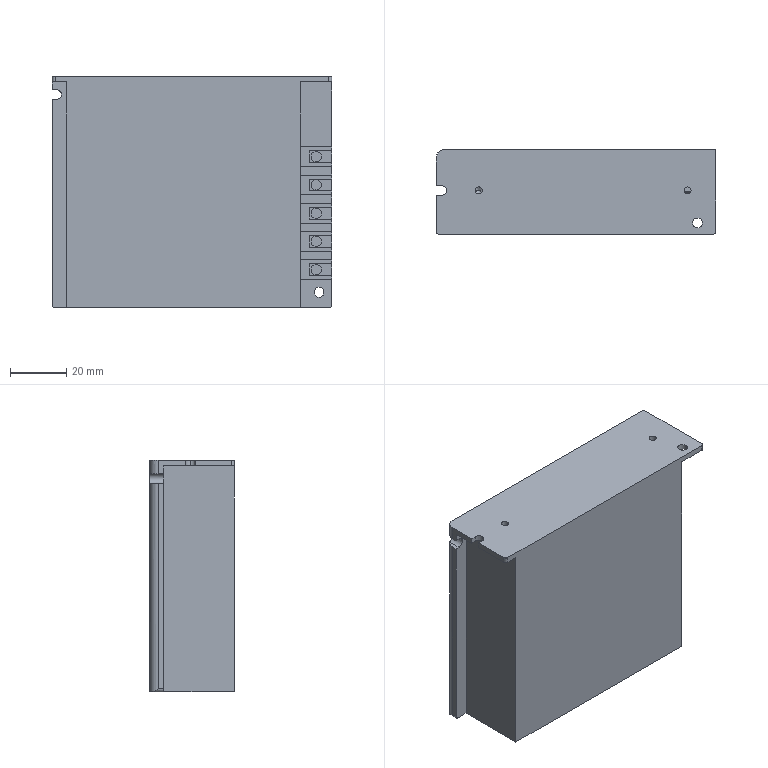Part | STEP file | Switching power supply LRS-50-24 (Mean Well) | 1 solid | 101 faces | box 99 x 30 x 82 mm | volume 213867 mm3 | plane 63 | cylinder 31 | cone 7 | commonest cylinder face diameters 3.666 x10 2.5 x8 2 x4 3.4 x4 3.5 x3 6 x2